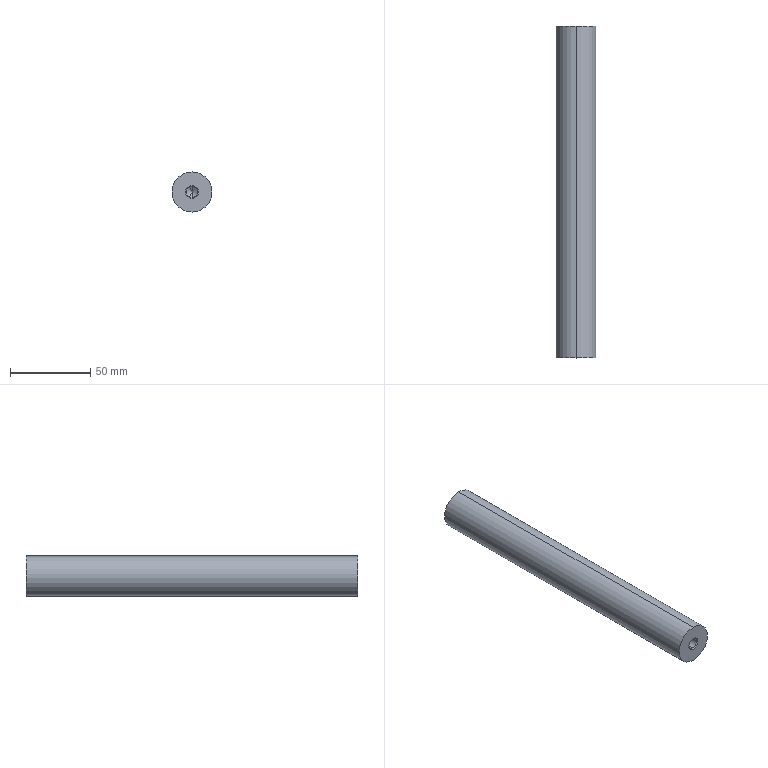Part | STEP file | A14-051 | 1 solid | 16 faces | box 25 x 207 x 25 mm | volume 99936 mm3 | cone 8 | cylinder 6 | plane 2 | commonest cylinder face diameters 6.8 x4 25 x2
STEP:
#1=CARTESIAN_POINT('',(0.,0.,0.));
#2=DIRECTION('',(0.,0.,1.));
#3=DIRECTION('',(1.,0.,0.));
#4=AXIS2_PLACEMENT_3D('',#1,#2,#3);
#5=CARTESIAN_POINT('',(0.,102.875,3.4));
#6=VERTEX_POINT('',#5);
#7=CARTESIAN_POINT('',(0.,103.5,4.025));
#8=VERTEX_POINT('',#7);
#9=CARTESIAN_POINT('',(0.,103.5,4.025));
#10=DIRECTION('',(0.,0.7071,0.7071));
#11=VECTOR('',#10,1.);
#12=LINE('',#9,#11);
#13=CARTESIAN_POINT('',(0.,103.5,0.));
#14=DIRECTION('',(0.,1.,0.));
#15=DIRECTION('',(0.,0.,1.));
#16=AXIS2_PLACEMENT_3D('',#13,#14,#15);
#17=CONICAL_SURFACE('',#16,4.025,0.7854);
#18=CARTESIAN_POINT('',(6.283,0.));
#19=DIRECTION('',(0.,1.));
#20=VECTOR('',#19,1.);
#21=LINE('',#18,#20);
#22=(GEOMETRIC_REPRESENTATION_CONTEXT(2)PARAMETRIC_REPRESENTATION_CONTEXT()REPRESENTATION_CONTEXT('',''));
#23=DEFINITIONAL_REPRESENTATION('',(#21),#22);
#24=PCURVE('',#17,#23);
#25=CARTESIAN_POINT('',(0.,103.5,0.));
#26=DIRECTION('',(0.,1.,0.));
#27=DIRECTION('',(0.,0.,1.));
#28=AXIS2_PLACEMENT_3D('',#25,#26,#27);
#29=CONICAL_SURFACE('',#28,4.025,0.7854);
#30=CARTESIAN_POINT('',(0.,0.));
#31=DIRECTION('',(0.,1.));
#32=VECTOR('',#31,1.);
#33=LINE('',#30,#32);
#34=(GEOMETRIC_REPRESENTATION_CONTEXT(2)PARAMETRIC_REPRESENTATION_CONTEXT()REPRESENTATION_CONTEXT('',''));
#35=DEFINITIONAL_REPRESENTATION('',(#33),#34);
#36=PCURVE('',#29,#35);
#37=SURFACE_CURVE('',#12,(#24,#36),.PCURVE_S1.);
#38=EDGE_CURVE('',#6,#8,#37,.T.);
#39=ORIENTED_EDGE('',*,*,#38,.T.);
#40=CARTESIAN_POINT('',(0.,103.5,-4.025));
#41=VERTEX_POINT('',#40);
#42=CARTESIAN_POINT('',(0.,103.5,0.));
#43=DIRECTION('',(0.,1.,0.));
#44=DIRECTION('',(0.,0.,1.));
#45=AXIS2_PLACEMENT_3D('',#42,#43,#44);
#46=CIRCLE('',#45,4.025);
#47=CARTESIAN_POINT('',(0.,0.));
#48=DIRECTION('',(1.,0.));
#49=VECTOR('',#48,1.);
#50=LINE('',#47,#49);
#51=(GEOMETRIC_REPRESENTATION_CONTEXT(2)PARAMETRIC_REPRESENTATION_CONTEXT()REPRESENTATION_CONTEXT('',''));
#52=DEFINITIONAL_REPRESENTATION('',(#50),#51);
#53=PCURVE('',#17,#52);
#54=CARTESIAN_POINT('',(0.,103.5,0.));
#55=DIRECTION('',(0.,1.,0.));
#56=DIRECTION('',(0.,0.,1.));
#57=AXIS2_PLACEMENT_3D('',#54,#55,#56);
#58=PLANE('',#57);
#59=CARTESIAN_POINT('',(0.,0.));
#60=DIRECTION('',(1.,0.));
#61=AXIS2_PLACEMENT_2D('',#59,#60);
#62=CIRCLE('',#61,4.025);
#63=(GEOMETRIC_REPRESENTATION_CONTEXT(2)PARAMETRIC_REPRESENTATION_CONTEXT()REPRESENTATION_CONTEXT('',''));
#64=DEFINITIONAL_REPRESENTATION('',(#62),#63);
#65=PCURVE('',#58,#64);
#66=SURFACE_CURVE('',#46,(#53,#65),.PCURVE_S1.);
#67=EDGE_CURVE('',#41,#8,#66,.T.);
#68=ORIENTED_EDGE('',*,*,#67,.F.);
#69=CARTESIAN_POINT('',(0.,102.875,-3.4));
#70=VERTEX_POINT('',#69);
#71=CARTESIAN_POINT('',(0.,103.5,-4.025));
#72=DIRECTION('',(0.,0.7071,-0.7071));
#73=VECTOR('',#72,1.);
#74=LINE('',#71,#73);
#75=CARTESIAN_POINT('',(3.142,0.));
#76=DIRECTION('',(0.,1.));
#77=VECTOR('',#76,1.);
#78=LINE('',#75,#77);
#79=(GEOMETRIC_REPRESENTATION_CONTEXT(2)PARAMETRIC_REPRESENTATION_CONTEXT()REPRESENTATION_CONTEXT('',''));
#80=DEFINITIONAL_REPRESENTATION('',(#78),#79);
#81=PCURVE('',#17,#80);
#82=CARTESIAN_POINT('',(3.142,0.));
#83=DIRECTION('',(0.,1.));
#84=VECTOR('',#83,1.);
#85=LINE('',#82,#84);
#86=(GEOMETRIC_REPRESENTATION_CONTEXT(2)PARAMETRIC_REPRESENTATION_CONTEXT()REPRESENTATION_CONTEXT('',''));
#87=DEFINITIONAL_REPRESENTATION('',(#85),#86);
#88=PCURVE('',#29,#87);
#89=SURFACE_CURVE('',#74,(#81,#88),.PCURVE_S1.);
#90=EDGE_CURVE('',#70,#41,#89,.T.);
#91=ORIENTED_EDGE('',*,*,#90,.F.);
#92=CARTESIAN_POINT('',(0.,102.875,0.));
#93=DIRECTION('',(0.,1.,0.));
#94=DIRECTION('',(0.,0.,1.));
#95=AXIS2_PLACEMENT_3D('',#92,#93,#94);
#96=CIRCLE('',#95,3.4);
#97=CARTESIAN_POINT('',(0.,-0.625));
#98=DIRECTION('',(1.,0.));
#99=VECTOR('',#98,1.);
#100=LINE('',#97,#99);
#101=(GEOMETRIC_REPRESENTATION_CONTEXT(2)PARAMETRIC_REPRESENTATION_CONTEXT()REPRESENTATION_CONTEXT('',''));
#102=DEFINITIONAL_REPRESENTATION('',(#100),#101);
#103=PCURVE('',#17,#102);
#104=CARTESIAN_POINT('',(0.,103.5,0.));
#105=DIRECTION('',(0.,1.,0.));
#106=DIRECTION('',(0.,0.,1.));
#107=AXIS2_PLACEMENT_3D('',#104,#105,#106);
#108=CYLINDRICAL_SURFACE('',#107,3.4);
#109=CARTESIAN_POINT('',(0.,-0.625));
#110=DIRECTION('',(1.,0.));
#111=VECTOR('',#110,1.);
#112=LINE('',#109,#111);
#113=(GEOMETRIC_REPRESENTATION_CONTEXT(2)PARAMETRIC_REPRESENTATION_CONTEXT()REPRESENTATION_CONTEXT('',''));
#114=DEFINITIONAL_REPRESENTATION('',(#112),#113);
#115=PCURVE('',#108,#114);
#116=SURFACE_CURVE('',#96,(#103,#115),.PCURVE_S1.);
#117=EDGE_CURVE('',#70,#6,#116,.T.);
#118=ORIENTED_EDGE('',*,*,#117,.T.);
#119=EDGE_LOOP('',(#39,#68,#91,#118));
#120=FACE_BOUND('',#119,.F.);
#121=ADVANCED_FACE('',(#120),#17,.F.);
#122=CARTESIAN_POINT('',(0.,81.25,3.4));
#123=VERTEX_POINT('',#122);
#124=CARTESIAN_POINT('',(0.,103.5,3.4));
#125=DIRECTION('',(0.,1.,0.));
#126=VECTOR('',#125,1.);
#127=LINE('',#124,#126);
#128=CARTESIAN_POINT('',(6.283,0.));
#129=DIRECTION('',(0.,1.));
#130=VECTOR('',#129,1.);
#131=LINE('',#128,#130);
#132=(GEOMETRIC_REPRESENTATION_CONTEXT(2)PARAMETRIC_REPRESENTATION_CONTEXT()REPRESENTATION_CONTEXT('',''));
#133=DEFINITIONAL_REPRESENTATION('',(#131),#132);
#134=PCURVE('',#108,#133);
#135=CARTESIAN_POINT('',(0.,103.5,0.));
#136=DIRECTION('',(0.,1.,0.));
#137=DIRECTION('',(0.,0.,1.));
#138=AXIS2_PLACEMENT_3D('',#135,#136,#137);
#139=CYLINDRICAL_SURFACE('',#138,3.4);
#140=CARTESIAN_POINT('',(0.,0.));
#141=DIRECTION('',(0.,1.));
#142=VECTOR('',#141,1.);
#143=LINE('',#140,#142);
#144=(GEOMETRIC_REPRESENTATION_CONTEXT(2)PARAMETRIC_REPRESENTATION_CONTEXT()REPRESENTATION_CONTEXT('',''));
#145=DEFINITIONAL_REPRESENTATION('',(#143),#144);
#146=PCURVE('',#139,#145);
#147=SURFACE_CURVE('',#127,(#134,#146),.PCURVE_S1.);
#148=EDGE_CURVE('',#123,#6,#147,.T.);
#149=ORIENTED_EDGE('',*,*,#148,.T.);
#150=ORIENTED_EDGE('',*,*,#117,.F.);
#151=CARTESIAN_POINT('',(0.,81.25,-3.4));
#152=VERTEX_POINT('',#151);
#153=CARTESIAN_POINT('',(0.,103.5,-3.4));
#154=DIRECTION('',(0.,1.,0.));
#155=VECTOR('',#154,1.);
#156=LINE('',#153,#155);
#157=CARTESIAN_POINT('',(3.142,0.));
#158=DIRECTION('',(0.,1.));
#159=VECTOR('',#158,1.);
#160=LINE('',#157,#159);
#161=(GEOMETRIC_REPRESENTATION_CONTEXT(2)PARAMETRIC_REPRESENTATION_CONTEXT()REPRESENTATION_CONTEXT('',''));
#162=DEFINITIONAL_REPRESENTATION('',(#160),#161);
#163=PCURVE('',#108,#162);
#164=CARTESIAN_POINT('',(3.142,0.));
#165=DIRECTION('',(0.,1.));
#166=VECTOR('',#165,1.);
#167=LINE('',#164,#166);
#168=(GEOMETRIC_REPRESENTATION_CONTEXT(2)PARAMETRIC_REPRESENTATION_CONTEXT()REPRESENTATION_CONTEXT('',''));
#169=DEFINITIONAL_REPRESENTATION('',(#167),#168);
#170=PCURVE('',#139,#169);
#171=SURFACE_CURVE('',#156,(#163,#170),.PCURVE_S1.);
#172=EDGE_CURVE('',#152,#70,#171,.T.);
#173=ORIENTED_EDGE('',*,*,#172,.F.);
#174=CARTESIAN_POINT('',(0.,81.25,0.));
#175=DIRECTION('',(0.,1.,0.));
#176=DIRECTION('',(0.,0.,1.));
#177=AXIS2_PLACEMENT_3D('',#174,#175,#176);
#178=CIRCLE('',#177,3.4);
#179=CARTESIAN_POINT('',(0.,-22.25));
#180=DIRECTION('',(1.,0.));
#181=VECTOR('',#180,1.);
#182=LINE('',#179,#181);
#183=(GEOMETRIC_REPRESENTATION_CONTEXT(2)PARAMETRIC_REPRESENTATION_CONTEXT()REPRESENTATION_CONTEXT('',''));
#184=DEFINITIONAL_REPRESENTATION('',(#182),#183);
#185=PCURVE('',#108,#184);
#186=CARTESIAN_POINT('',(0.,81.25,0.));
#187=DIRECTION('',(0.,1.,0.));
#188=DIRECTION('',(0.,0.,1.));
#189=AXIS2_PLACEMENT_3D('',#186,#187,#188);
#190=CONICAL_SURFACE('',#189,3.4,1.03);
#191=CARTESIAN_POINT('',(0.,0.));
#192=DIRECTION('',(1.,0.));
#193=VECTOR('',#192,1.);
#194=LINE('',#191,#193);
#195=(GEOMETRIC_REPRESENTATION_CONTEXT(2)PARAMETRIC_REPRESENTATION_CONTEXT()REPRESENTATION_CONTEXT('',''));
#196=DEFINITIONAL_REPRESENTATION('',(#194),#195);
#197=PCURVE('',#190,#196);
#198=SURFACE_CURVE('',#178,(#185,#197),.PCURVE_S1.);
#199=EDGE_CURVE('',#152,#123,#198,.T.);
#200=ORIENTED_EDGE('',*,*,#199,.T.);
#201=EDGE_LOOP('',(#149,#150,#173,#200));
#202=FACE_BOUND('',#201,.F.);
#203=ADVANCED_FACE('',(#202),#108,.F.);
#204=ORIENTED_EDGE('',*,*,#199,.F.);
#205=CARTESIAN_POINT('',(0.,79.207,0.));
#206=VERTEX_POINT('',#205);
#207=CARTESIAN_POINT('',(0.,81.25,-3.4));
#208=DIRECTION('',(0.,0.515,-0.8572));
#209=VECTOR('',#208,1.);
#210=LINE('',#207,#209);
#211=CARTESIAN_POINT('',(3.142,-2.043));
#212=CARTESIAN_POINT('',(3.142,-2.012));
#213=CARTESIAN_POINT('',(3.142,-1.95));
#214=CARTESIAN_POINT('',(3.142,-1.857));
#215=CARTESIAN_POINT('',(3.142,-1.764));
#216=CARTESIAN_POINT('',(3.142,-1.671));
#217=CARTESIAN_POINT('',(3.142,-1.579));
#218=CARTESIAN_POINT('',(3.142,-1.486));
#219=CARTESIAN_POINT('',(3.142,-1.393));
#220=CARTESIAN_POINT('',(3.142,-1.3));
#221=CARTESIAN_POINT('',(3.142,-1.207));
#222=CARTESIAN_POINT('',(3.142,-1.114));
#223=CARTESIAN_POINT('',(3.142,-1.021));
#224=CARTESIAN_POINT('',(3.142,-0.9286));
#225=CARTESIAN_POINT('',(3.142,-0.8357));
#226=CARTESIAN_POINT('',(3.142,-0.7429));
#227=CARTESIAN_POINT('',(3.142,-0.65));
#228=CARTESIAN_POINT('',(3.142,-0.5572));
#229=CARTESIAN_POINT('',(3.142,-0.4643));
#230=CARTESIAN_POINT('',(3.142,-0.3714));
#231=CARTESIAN_POINT('',(3.142,-0.2786));
#232=CARTESIAN_POINT('',(3.142,-0.1857));
#233=CARTESIAN_POINT('',(3.142,-0.09286));
#234=CARTESIAN_POINT('',(3.142,-0.03095));
#235=CARTESIAN_POINT('',(3.142,0.));
#236=B_SPLINE_CURVE_WITH_KNOTS('',3,(#211,#212,#213,#214,#215,#216,#217,#218,#219,#220,#221,#222,#223,#224,#225,#226,#227,#228,#229,#230,#231,#232,#233,#234,#235),.UNSPECIFIED.,.F.,.F.,(4,1,1,1,1,1,1,1,1,1,1,1,1,1,1,1,1,1,1,1,1,1,4),(-3.967,-3.786,-3.606,-3.426,-3.245,-3.065,-2.885,-2.704,-2.524,-2.344,-2.164,-1.983,-1.803,-1.623,-1.442,-1.262,-1.082,-0.9015,-0.7212,-0.5409,-0.3606,-0.1803,0.),.UNSPECIFIED.);
#237=(GEOMETRIC_REPRESENTATION_CONTEXT(2)PARAMETRIC_REPRESENTATION_CONTEXT()REPRESENTATION_CONTEXT('',''));
#238=DEFINITIONAL_REPRESENTATION('',(#236),#237);
#239=PCURVE('',#190,#238);
#240=CARTESIAN_POINT('',(0.,81.25,0.));
#241=DIRECTION('',(0.,1.,0.));
#242=DIRECTION('',(0.,0.,1.));
#243=AXIS2_PLACEMENT_3D('',#240,#241,#242);
#244=CONICAL_SURFACE('',#243,3.4,1.03);
#245=CARTESIAN_POINT('',(3.142,-2.043));
#246=CARTESIAN_POINT('',(3.142,-2.012));
#247=CARTESIAN_POINT('',(3.142,-1.95));
#248=CARTESIAN_POINT('',(3.142,-1.857));
#249=CARTESIAN_POINT('',(3.142,-1.764));
#250=CARTESIAN_POINT('',(3.142,-1.671));
#251=CARTESIAN_POINT('',(3.142,-1.579));
#252=CARTESIAN_POINT('',(3.142,-1.486));
#253=CARTESIAN_POINT('',(3.142,-1.393));
#254=CARTESIAN_POINT('',(3.142,-1.3));
#255=CARTESIAN_POINT('',(3.142,-1.207));
#256=CARTESIAN_POINT('',(3.142,-1.114));
#257=CARTESIAN_POINT('',(3.142,-1.021));
#258=CARTESIAN_POINT('',(3.142,-0.9286));
#259=CARTESIAN_POINT('',(3.142,-0.8357));
#260=CARTESIAN_POINT('',(3.142,-0.7429));
#261=CARTESIAN_POINT('',(3.142,-0.65));
#262=CARTESIAN_POINT('',(3.142,-0.5572));
#263=CARTESIAN_POINT('',(3.142,-0.4643));
#264=CARTESIAN_POINT('',(3.142,-0.3714));
#265=CARTESIAN_POINT('',(3.142,-0.2786));
#266=CARTESIAN_POINT('',(3.142,-0.1857));
#267=CARTESIAN_POINT('',(3.142,-0.09286));
#268=CARTESIAN_POINT('',(3.142,-0.03095));
#269=CARTESIAN_POINT('',(3.142,0.));
#270=B_SPLINE_CURVE_WITH_KNOTS('',3,(#245,#246,#247,#248,#249,#250,#251,#252,#253,#254,#255,#256,#257,#258,#259,#260,#261,#262,#263,#264,#265,#266,#267,#268,#269),.UNSPECIFIED.,.F.,.F.,(4,1,1,1,1,1,1,1,1,1,1,1,1,1,1,1,1,1,1,1,1,1,4),(-3.967,-3.786,-3.606,-3.426,-3.245,-3.065,-2.885,-2.704,-2.524,-2.344,-2.164,-1.983,-1.803,-1.623,-1.442,-1.262,-1.082,-0.9015,-0.7212,-0.5409,-0.3606,-0.1803,0.),.UNSPECIFIED.);
#271=(GEOMETRIC_REPRESENTATION_CONTEXT(2)PARAMETRIC_REPRESENTATION_CONTEXT()REPRESENTATION_CONTEXT('',''));
#272=DEFINITIONAL_REPRESENTATION('',(#270),#271);
#273=PCURVE('',#244,#272);
#274=SURFACE_CURVE('',#210,(#239,#273),.PCURVE_S1.);
#275=EDGE_CURVE('',#206,#152,#274,.T.);
#276=ORIENTED_EDGE('',*,*,#275,.F.);
#277=CARTESIAN_POINT('',(0.,81.25,3.4));
#278=DIRECTION('',(0.,0.515,0.8572));
#279=VECTOR('',#278,1.);
#280=LINE('',#277,#279);
#281=CARTESIAN_POINT('',(6.283,-2.043));
#282=CARTESIAN_POINT('',(6.283,-2.012));
#283=CARTESIAN_POINT('',(6.283,-1.95));
#284=CARTESIAN_POINT('',(6.283,-1.857));
#285=CARTESIAN_POINT('',(6.283,-1.764));
#286=CARTESIAN_POINT('',(6.283,-1.671));
#287=CARTESIAN_POINT('',(6.283,-1.579));
#288=CARTESIAN_POINT('',(6.283,-1.486));
#289=CARTESIAN_POINT('',(6.283,-1.393));
#290=CARTESIAN_POINT('',(6.283,-1.3));
#291=CARTESIAN_POINT('',(6.283,-1.207));
#292=CARTESIAN_POINT('',(6.283,-1.114));
#293=CARTESIAN_POINT('',(6.283,-1.021));
#294=CARTESIAN_POINT('',(6.283,-0.9286));
#295=CARTESIAN_POINT('',(6.283,-0.8357));
#296=CARTESIAN_POINT('',(6.283,-0.7429));
#297=CARTESIAN_POINT('',(6.283,-0.65));
#298=CARTESIAN_POINT('',(6.283,-0.5572));
#299=CARTESIAN_POINT('',(6.283,-0.4643));
#300=CARTESIAN_POINT('',(6.283,-0.3714));
#301=CARTESIAN_POINT('',(6.283,-0.2786));
#302=CARTESIAN_POINT('',(6.283,-0.1857));
#303=CARTESIAN_POINT('',(6.283,-0.09286));
#304=CARTESIAN_POINT('',(6.283,-0.03095));
#305=CARTESIAN_POINT('',(6.283,0.));
#306=B_SPLINE_CURVE_WITH_KNOTS('',3,(#281,#282,#283,#284,#285,#286,#287,#288,#289,#290,#291,#292,#293,#294,#295,#296,#297,#298,#299,#300,#301,#302,#303,#304,#305),.UNSPECIFIED.,.F.,.F.,(4,1,1,1,1,1,1,1,1,1,1,1,1,1,1,1,1,1,1,1,1,1,4),(-3.967,-3.786,-3.606,-3.426,-3.245,-3.065,-2.885,-2.704,-2.524,-2.344,-2.164,-1.983,-1.803,-1.623,-1.442,-1.262,-1.082,-0.9015,-0.7212,-0.5409,-0.3606,-0.1803,0.),.UNSPECIFIED.);
#307=(GEOMETRIC_REPRESENTATION_CONTEXT(2)PARAMETRIC_REPRESENTATION_CONTEXT()REPRESENTATION_CONTEXT('',''));
#308=DEFINITIONAL_REPRESENTATION('',(#306),#307);
#309=PCURVE('',#190,#308);
#310=CARTESIAN_POINT('',(0.,-2.043));
#311=CARTESIAN_POINT('',(0.,-2.012));
#312=CARTESIAN_POINT('',(0.,-1.95));
#313=CARTESIAN_POINT('',(0.,-1.857));
#314=CARTESIAN_POINT('',(0.,-1.764));
#315=CARTESIAN_POINT('',(0.,-1.671));
#316=CARTESIAN_POINT('',(0.,-1.579));
#317=CARTESIAN_POINT('',(0.,-1.486));
#318=CARTESIAN_POINT('',(0.,-1.393));
#319=CARTESIAN_POINT('',(0.,-1.3));
#320=CARTESIAN_POINT('',(0.,-1.207));
#321=CARTESIAN_POINT('',(0.,-1.114));
#322=CARTESIAN_POINT('',(0.,-1.021));
#323=CARTESIAN_POINT('',(0.,-0.9286));
#324=CARTESIAN_POINT('',(0.,-0.8357));
#325=CARTESIAN_POINT('',(0.,-0.7429));
#326=CARTESIAN_POINT('',(0.,-0.65));
#327=CARTESIAN_POINT('',(0.,-0.5572));
#328=CARTESIAN_POINT('',(0.,-0.4643));
#329=CARTESIAN_POINT('',(0.,-0.3714));
#330=CARTESIAN_POINT('',(0.,-0.2786));
#331=CARTESIAN_POINT('',(0.,-0.1857));
#332=CARTESIAN_POINT('',(0.,-0.09286));
#333=CARTESIAN_POINT('',(0.,-0.03095));
#334=CARTESIAN_POINT('',(0.,0.));
#335=B_SPLINE_CURVE_WITH_KNOTS('',3,(#310,#311,#312,#313,#314,#315,#316,#317,#318,#319,#320,#321,#322,#323,#324,#325,#326,#327,#328,#329,#330,#331,#332,#333,#334),.UNSPECIFIED.,.F.,.F.,(4,1,1,1,1,1,1,1,1,1,1,1,1,1,1,1,1,1,1,1,1,1,4),(-3.967,-3.786,-3.606,-3.426,-3.245,-3.065,-2.885,-2.704,-2.524,-2.344,-2.164,-1.983,-1.803,-1.623,-1.442,-1.262,-1.082,-0.9015,-0.7212,-0.5409,-0.3606,-0.1803,0.),.UNSPECIFIED.);
#336=(GEOMETRIC_REPRESENTATION_CONTEXT(2)PARAMETRIC_REPRESENTATION_CONTEXT()REPRESENTATION_CONTEXT('',''));
#337=DEFINITIONAL_REPRESENTATION('',(#335),#336);
#338=PCURVE('',#244,#337);
#339=SURFACE_CURVE('',#280,(#309,#338),.PCURVE_S1.);
#340=EDGE_CURVE('',#206,#123,#339,.T.);
#341=ORIENTED_EDGE('',*,*,#340,.T.);
#342=EDGE_LOOP('',(#204,#276,#341));
#343=FACE_BOUND('',#342,.F.);
#344=ADVANCED_FACE('',(#343),#190,.F.);
#345=CARTESIAN_POINT('',(0.,-102.875,-3.4));
#346=VERTEX_POINT('',#345);
#347=CARTESIAN_POINT('',(0.,-103.5,-4.025));
#348=VERTEX_POINT('',#347);
#349=CARTESIAN_POINT('',(0.,-103.5,-4.025));
#350=DIRECTION('',(0.,-0.7071,-0.7071));
#351=VECTOR('',#350,1.);
#352=LINE('',#349,#351);
#353=CARTESIAN_POINT('',(0.,-103.5,0.));
#354=DIRECTION('',(0.,-1.,0.));
#355=DIRECTION('',(0.,0.,-1.));
#356=AXIS2_PLACEMENT_3D('',#353,#354,#355);
#357=CONICAL_SURFACE('',#356,4.025,0.7854);
#358=CARTESIAN_POINT('',(6.283,0.));
#359=DIRECTION('',(0.,1.));
#360=VECTOR('',#359,1.);
#361=LINE('',#358,#360);
#362=(GEOMETRIC_REPRESENTATION_CONTEXT(2)PARAMETRIC_REPRESENTATION_CONTEXT()REPRESENTATION_CONTEXT('',''));
#363=DEFINITIONAL_REPRESENTATION('',(#361),#362);
#364=PCURVE('',#357,#363);
#365=CARTESIAN_POINT('',(0.,-103.5,0.));
#366=DIRECTION('',(0.,-1.,0.));
#367=DIRECTION('',(0.,0.,-1.));
#368=AXIS2_PLACEMENT_3D('',#365,#366,#367);
#369=CONICAL_SURFACE('',#368,4.025,0.7854);
#370=CARTESIAN_POINT('',(0.,0.));
#371=DIRECTION('',(0.,1.));
#372=VECTOR('',#371,1.);
#373=LINE('',#370,#372);
#374=(GEOMETRIC_REPRESENTATION_CONTEXT(2)PARAMETRIC_REPRESENTATION_CONTEXT()REPRESENTATION_CONTEXT('',''));
#375=DEFINITIONAL_REPRESENTATION('',(#373),#374);
#376=PCURVE('',#369,#375);
#377=SURFACE_CURVE('',#352,(#364,#376),.PCURVE_S1.);
#378=EDGE_CURVE('',#346,#348,#377,.T.);
#379=ORIENTED_EDGE('',*,*,#378,.T.);
#380=CARTESIAN_POINT('',(0.,-103.5,4.025));
#381=VERTEX_POINT('',#380);
#382=CARTESIAN_POINT('',(0.,-103.5,0.));
#383=DIRECTION('',(0.,-1.,0.));
#384=DIRECTION('',(0.,0.,-1.));
#385=AXIS2_PLACEMENT_3D('',#382,#383,#384);
#386=CIRCLE('',#385,4.025);
#387=CARTESIAN_POINT('',(0.,0.));
#388=DIRECTION('',(1.,0.));
#389=VECTOR('',#388,1.);
#390=LINE('',#387,#389);
#391=(GEOMETRIC_REPRESENTATION_CONTEXT(2)PARAMETRIC_REPRESENTATION_CONTEXT()REPRESENTATION_CONTEXT('',''));
#392=DEFINITIONAL_REPRESENTATION('',(#390),#391);
#393=PCURVE('',#357,#392);
#394=CARTESIAN_POINT('',(0.,-103.5,0.));
#395=DIRECTION('',(0.,1.,0.));
#396=DIRECTION('',(0.,0.,1.));
#397=AXIS2_PLACEMENT_3D('',#394,#395,#396);
#398=PLANE('',#397);
#399=CARTESIAN_POINT('',(-4.025,0.));
#400=CARTESIAN_POINT('',(-4.025,6.972));
#401=CARTESIAN_POINT('',(2.013,3.486));
#402=CARTESIAN_POINT('',(8.05,0.));
#403=CARTESIAN_POINT('',(2.013,-3.486));
#404=CARTESIAN_POINT('',(-4.025,-6.972));
#405=CARTESIAN_POINT('',(-4.025,0.));
#406=(BOUNDED_CURVE()B_SPLINE_CURVE(2,(#399,#400,#401,#402,#403,#404,#405),.UNSPECIFIED.,.T.,.F.)B_SPLINE_CURVE_WITH_KNOTS((1,2,2,2,2,1),(-2.094,0.,2.094,4.189,6.283,8.378),.UNSPECIFIED.)CURVE()GEOMETRIC_REPRESENTATION_ITEM()RATIONAL_B_SPLINE_CURVE((1.,0.5,1.,0.5,1.,0.5,1.))REPRESENTATION_ITEM(''));
#407=(GEOMETRIC_REPRESENTATION_CONTEXT(2)PARAMETRIC_REPRESENTATION_CONTEXT()REPRESENTATION_CONTEXT('',''));
#408=DEFINITIONAL_REPRESENTATION('',(#406),#407);
#409=PCURVE('',#398,#408);
#410=SURFACE_CURVE('',#386,(#393,#409),.PCURVE_S1.);
#411=EDGE_CURVE('',#381,#348,#410,.T.);
#412=ORIENTED_EDGE('',*,*,#411,.F.);
#413=CARTESIAN_POINT('',(0.,-102.875,3.4));
#414=VERTEX_POINT('',#413);
#415=CARTESIAN_POINT('',(0.,-103.5,4.025));
#416=DIRECTION('',(0.,-0.7071,0.7071));
#417=VECTOR('',#416,1.);
#418=LINE('',#415,#417);
#419=CARTESIAN_POINT('',(3.142,0.));
#420=DIRECTION('',(0.,1.));
#421=VECTOR('',#420,1.);
#422=LINE('',#419,#421);
#423=(GEOMETRIC_REPRESENTATION_CONTEXT(2)PARAMETRIC_REPRESENTATION_CONTEXT()REPRESENTATION_CONTEXT('',''));
#424=DEFINITIONAL_REPRESENTATION('',(#422),#423);
#425=PCURVE('',#357,#424);
#426=CARTESIAN_POINT('',(3.142,0.));
#427=DIRECTION('',(0.,1.));
#428=VECTOR('',#427,1.);
#429=LINE('',#426,#428);
#430=(GEOMETRIC_REPRESENTATION_CONTEXT(2)PARAMETRIC_REPRESENTATION_CONTEXT()REPRESENTATION_CONTEXT('',''));
#431=DEFINITIONAL_REPRESENTATION('',(#429),#430);
#432=PCURVE('',#369,#431);
#433=SURFACE_CURVE('',#418,(#425,#432),.PCURVE_S1.);
#434=EDGE_CURVE('',#414,#381,#433,.T.);
#435=ORIENTED_EDGE('',*,*,#434,.F.);
#436=CARTESIAN_POINT('',(0.,-102.875,0.));
#437=DIRECTION('',(0.,-1.,0.));
#438=DIRECTION('',(0.,0.,-1.));
#439=AXIS2_PLACEMENT_3D('',#436,#437,#438);
#440=CIRCLE('',#439,3.4);
#441=CARTESIAN_POINT('',(0.,-0.625));
#442=DIRECTION('',(1.,0.));
#443=VECTOR('',#442,1.);
#444=LINE('',#441,#443);
#445=(GEOMETRIC_REPRESENTATION_CONTEXT(2)PARAMETRIC_REPRESENTATION_CONTEXT()REPRESENTATION_CONTEXT('',''));
#446=DEFINITIONAL_REPRESENTATION('',(#444),#445);
#447=PCURVE('',#357,#446);
#448=CARTESIAN_POINT('',(0.,-103.5,0.));
#449=DIRECTION('',(0.,-1.,0.));
#450=DIRECTION('',(0.,0.,-1.));
#451=AXIS2_PLACEMENT_3D('',#448,#449,#450);
#452=CYLINDRICAL_SURFACE('',#451,3.4);
#453=CARTESIAN_POINT('',(0.,-0.625));
#454=DIRECTION('',(1.,0.));
#455=VECTOR('',#454,1.);
#456=LINE('',#453,#455);
#457=(GEOMETRIC_REPRESENTATION_CONTEXT(2)PARAMETRIC_REPRESENTATION_CONTEXT()REPRESENTATION_CONTEXT('',''));
#458=DEFINITIONAL_REPRESENTATION('',(#456),#457);
#459=PCURVE('',#452,#458);
#460=SURFACE_CURVE('',#440,(#447,#459),.PCURVE_S1.);
#461=EDGE_CURVE('',#414,#346,#460,.T.);
#462=ORIENTED_EDGE('',*,*,#461,.T.);
#463=EDGE_LOOP('',(#379,#412,#435,#462));
#464=FACE_BOUND('',#463,.F.);
#465=ADVANCED_FACE('',(#464),#357,.F.);
#466=CARTESIAN_POINT('',(0.,-81.25,-3.4));
#467=VERTEX_POINT('',#466);
#468=CARTESIAN_POINT('',(0.,-103.5,-3.4));
#469=DIRECTION('',(0.,-1.,0.));
#470=VECTOR('',#469,1.);
#471=LINE('',#468,#470);
#472=CARTESIAN_POINT('',(6.283,0.));
#473=DIRECTION('',(0.,1.));
#474=VECTOR('',#473,1.);
#475=LINE('',#472,#474);
#476=(GEOMETRIC_REPRESENTATION_CONTEXT(2)PARAMETRIC_REPRESENTATION_CONTEXT()REPRESENTATION_CONTEXT('',''));
#477=DEFINITIONAL_REPRESENTATION('',(#475),#476);
#478=PCURVE('',#452,#477);
#479=CARTESIAN_POINT('',(0.,-103.5,0.));
#480=DIRECTION('',(0.,-1.,0.));
#481=DIRECTION('',(0.,0.,-1.));
#482=AXIS2_PLACEMENT_3D('',#479,#480,#481);
#483=CYLINDRICAL_SURFACE('',#482,3.4);
#484=CARTESIAN_POINT('',(0.,0.));
#485=DIRECTION('',(0.,1.));
#486=VECTOR('',#485,1.);
#487=LINE('',#484,#486);
#488=(GEOMETRIC_REPRESENTATION_CONTEXT(2)PARAMETRIC_REPRESENTATION_CONTEXT()REPRESENTATION_CONTEXT('',''));
#489=DEFINITIONAL_REPRESENTATION('',(#487),#488);
#490=PCURVE('',#483,#489);
#491=SURFACE_CURVE('',#471,(#478,#490),.PCURVE_S1.);
#492=EDGE_CURVE('',#467,#346,#491,.T.);
#493=ORIENTED_EDGE('',*,*,#492,.T.);
#494=ORIENTED_EDGE('',*,*,#461,.F.);
#495=CARTESIAN_POINT('',(0.,-81.25,3.4));
#496=VERTEX_POINT('',#495);
#497=CARTESIAN_POINT('',(0.,-103.5,3.4));
#498=DIRECTION('',(0.,-1.,0.));
#499=VECTOR('',#498,1.);
#500=LINE('',#497,#499);
#501=CARTESIAN_POINT('',(3.142,0.));
#502=DIRECTION('',(0.,1.));
#503=VECTOR('',#502,1.);
#504=LINE('',#501,#503);
#505=(GEOMETRIC_REPRESENTATION_CONTEXT(2)PARAMETRIC_REPRESENTATION_CONTEXT()REPRESENTATION_CONTEXT('',''));
#506=DEFINITIONAL_REPRESENTATION('',(#504),#505);
#507=PCURVE('',#452,#506);
#508=CARTESIAN_POINT('',(3.142,0.));
#509=DIRECTION('',(0.,1.));
#510=VECTOR('',#509,1.);
#511=LINE('',#508,#510);
#512=(GEOMETRIC_REPRESENTATION_CONTEXT(2)PARAMETRIC_REPRESENTATION_CONTEXT()REPRESENTATION_CONTEXT('',''));
#513=DEFINITIONAL_REPRESENTATION('',(#511),#512);
#514=PCURVE('',#483,#513);
#515=SURFACE_CURVE('',#500,(#507,#514),.PCURVE_S1.);
#516=EDGE_CURVE('',#496,#414,#515,.T.);
#517=ORIENTED_EDGE('',*,*,#516,.F.);
#518=CARTESIAN_POINT('',(0.,-81.25,0.));
#519=DIRECTION('',(0.,-1.,0.));
#520=DIRECTION('',(0.,0.,-1.));
#521=AXIS2_PLACEMENT_3D('',#518,#519,#520);
#522=CIRCLE('',#521,3.4);
#523=CARTESIAN_POINT('',(0.,-22.25));
#524=DIRECTION('',(1.,0.));
#525=VECTOR('',#524,1.);
#526=LINE('',#523,#525);
#527=(GEOMETRIC_REPRESENTATION_CONTEXT(2)PARAMETRIC_REPRESENTATION_CONTEXT()REPRESENTATION_CONTEXT('',''));
#528=DEFINITIONAL_REPRESENTATION('',(#526),#527);
#529=PCURVE('',#452,#528);
#530=CARTESIAN_POINT('',(0.,-81.25,0.));
#531=DIRECTION('',(0.,-1.,0.));
#532=DIRECTION('',(0.,0.,-1.));
#533=AXIS2_PLACEMENT_3D('',#530,#531,#532);
#534=CONICAL_SURFACE('',#533,3.4,1.03);
#535=CARTESIAN_POINT('',(0.,0.));
#536=DIRECTION('',(1.,0.));
#537=VECTOR('',#536,1.);
#538=LINE('',#535,#537);
#539=(GEOMETRIC_REPRESENTATION_CONTEXT(2)PARAMETRIC_REPRESENTATION_CONTEXT()REPRESENTATION_CONTEXT('',''));
#540=DEFINITIONAL_REPRESENTATION('',(#538),#539);
#541=PCURVE('',#534,#540);
#542=SURFACE_CURVE('',#522,(#529,#541),.PCURVE_S1.);
#543=EDGE_CURVE('',#496,#467,#542,.T.);
#544=ORIENTED_EDGE('',*,*,#543,.T.);
#545=EDGE_LOOP('',(#493,#494,#517,#544));
#546=FACE_BOUND('',#545,.F.);
#547=ADVANCED_FACE('',(#546),#452,.F.);
#548=ORIENTED_EDGE('',*,*,#543,.F.);
#549=CARTESIAN_POINT('',(0.,-79.207,0.));
#550=VERTEX_POINT('',#549);
#551=CARTESIAN_POINT('',(0.,-81.25,3.4));
#552=DIRECTION('',(0.,-0.515,0.8572));
#553=VECTOR('',#552,1.);
#554=LINE('',#551,#553);
#555=CARTESIAN_POINT('',(3.142,-2.043));
#556=CARTESIAN_POINT('',(3.142,-2.012));
#557=CARTESIAN_POINT('',(3.142,-1.95));
#558=CARTESIAN_POINT('',(3.142,-1.857));
#559=CARTESIAN_POINT('',(3.142,-1.764));
#560=CARTESIAN_POINT('',(3.142,-1.671));
#561=CARTESIAN_POINT('',(3.142,-1.579));
#562=CARTESIAN_POINT('',(3.142,-1.486));
#563=CARTESIAN_POINT('',(3.142,-1.393));
#564=CARTESIAN_POINT('',(3.142,-1.3));
#565=CARTESIAN_POINT('',(3.142,-1.207));
#566=CARTESIAN_POINT('',(3.142,-1.114));
#567=CARTESIAN_POINT('',(3.142,-1.021));
#568=CARTESIAN_POINT('',(3.142,-0.9286));
#569=CARTESIAN_POINT('',(3.142,-0.8357));
#570=CARTESIAN_POINT('',(3.142,-0.7429));
#571=CARTESIAN_POINT('',(3.142,-0.65));
#572=CARTESIAN_POINT('',(3.142,-0.5572));
#573=CARTESIAN_POINT('',(3.142,-0.4643));
#574=CARTESIAN_POINT('',(3.142,-0.3714));
#575=CARTESIAN_POINT('',(3.142,-0.2786));
#576=CARTESIAN_POINT('',(3.142,-0.1857));
#577=CARTESIAN_POINT('',(3.142,-0.09286));
#578=CARTESIAN_POINT('',(3.142,-0.03095));
#579=CARTESIAN_POINT('',(3.142,0.));
#580=B_SPLINE_CURVE_WITH_KNOTS('',3,(#555,#556,#557,#558,#559,#560,#561,#562,#563,#564,#565,#566,#567,#568,#569,#570,#571,#572,#573,#574,#575,#576,#577,#578,#579),.UNSPECIFIED.,.F.,.F.,(4,1,1,1,1,1,1,1,1,1,1,1,1,1,1,1,1,1,1,1,1,1,4),(-3.967,-3.786,-3.606,-3.426,-3.245,-3.065,-2.885,-2.704,-2.524,-2.344,-2.164,-1.983,-1.803,-1.623,-1.442,-1.262,-1.082,-0.9015,-0.7212,-0.5409,-0.3606,-0.1803,0.),.UNSPECIFIED.);
#581=(GEOMETRIC_REPRESENTATION_CONTEXT(2)PARAMETRIC_REPRESENTATION_CONTEXT()REPRESENTATION_CONTEXT('',''));
#582=DEFINITIONAL_REPRESENTATION('',(#580),#581);
#583=PCURVE('',#534,#582);
#584=CARTESIAN_POINT('',(0.,-81.25,0.));
#585=DIRECTION('',(0.,-1.,0.));
#586=DIRECTION('',(0.,0.,-1.));
#587=AXIS2_PLACEMENT_3D('',#584,#585,#586);
#588=CONICAL_SURFACE('',#587,3.4,1.03);
#589=CARTESIAN_POINT('',(3.142,-2.043));
#590=CARTESIAN_POINT('',(3.142,-2.012));
#591=CARTESIAN_POINT('',(3.142,-1.95));
#592=CARTESIAN_POINT('',(3.142,-1.857));
#593=CARTESIAN_POINT('',(3.142,-1.764));
#594=CARTESIAN_POINT('',(3.142,-1.671));
#595=CARTESIAN_POINT('',(3.142,-1.579));
#596=CARTESIAN_POINT('',(3.142,-1.486));
#597=CARTESIAN_POINT('',(3.142,-1.393));
#598=CARTESIAN_POINT('',(3.142,-1.3));
#599=CARTESIAN_POINT('',(3.142,-1.207));
#600=CARTESIAN_POINT('',(3.142,-1.114));
#601=CARTESIAN_POINT('',(3.142,-1.021));
#602=CARTESIAN_POINT('',(3.142,-0.9286));
#603=CARTESIAN_POINT('',(3.142,-0.8357));
#604=CARTESIAN_POINT('',(3.142,-0.7429));
#605=CARTESIAN_POINT('',(3.142,-0.65));
#606=CARTESIAN_POINT('',(3.142,-0.5572));
#607=CARTESIAN_POINT('',(3.142,-0.4643));
#608=CARTESIAN_POINT('',(3.142,-0.3714));
#609=CARTESIAN_POINT('',(3.142,-0.2786));
#610=CARTESIAN_POINT('',(3.142,-0.1857));
#611=CARTESIAN_POINT('',(3.142,-0.09286));
#612=CARTESIAN_POINT('',(3.142,-0.03095));
#613=CARTESIAN_POINT('',(3.142,0.));
#614=B_SPLINE_CURVE_WITH_KNOTS('',3,(#589,#590,#591,#592,#593,#594,#595,#596,#597,#598,#599,#600,#601,#602,#603,#604,#605,#606,#607,#608,#609,#610,#611,#612,#613),.UNSPECIFIED.,.F.,.F.,(4,1,1,1,1,1,1,1,1,1,1,1,1,1,1,1,1,1,1,1,1,1,4),(-3.967,-3.786,-3.606,-3.426,-3.245,-3.065,-2.885,-2.704,-2.524,-2.344,-2.164,-1.983,-1.803,-1.623,-1.442,-1.262,-1.082,-0.9015,-0.7212,-0.5409,-0.3606,-0.1803,0.),.UNSPECIFIED.);
#615=(GEOMETRIC_REPRESENTATION_CONTEXT(2)PARAMETRIC_REPRESENTATION_CONTEXT()REPRESENTATION_CONTEXT('',''));
#616=DEFINITIONAL_REPRESENTATION('',(#614),#615);
#617=PCURVE('',#588,#616);
#618=SURFACE_CURVE('',#554,(#583,#617),.PCURVE_S1.);
#619=EDGE_CURVE('',#550,#496,#618,.T.);
#620=ORIENTED_EDGE('',*,*,#619,.F.);
#621=CARTESIAN_POINT('',(0.,-81.25,-3.4));
#622=DIRECTION('',(0.,-0.515,-0.8572));
#623=VECTOR('',#622,1.);
#624=LINE('',#621,#623);
#625=CARTESIAN_POINT('',(6.283,-2.043));
#626=CARTESIAN_POINT('',(6.283,-2.012));
#627=CARTESIAN_POINT('',(6.283,-1.95));
#628=CARTESIAN_POINT('',(6.283,-1.857));
#629=CARTESIAN_POINT('',(6.283,-1.764));
#630=CARTESIAN_POINT('',(6.283,-1.671));
#631=CARTESIAN_POINT('',(6.283,-1.579));
#632=CARTESIAN_POINT('',(6.283,-1.486));
#633=CARTESIAN_POINT('',(6.283,-1.393));
#634=CARTESIAN_POINT('',(6.283,-1.3));
#635=CARTESIAN_POINT('',(6.283,-1.207));
#636=CARTESIAN_POINT('',(6.283,-1.114));
#637=CARTESIAN_POINT('',(6.283,-1.021));
#638=CARTESIAN_POINT('',(6.283,-0.9286));
#639=CARTESIAN_POINT('',(6.283,-0.8357));
#640=CARTESIAN_POINT('',(6.283,-0.7429));
#641=CARTESIAN_POINT('',(6.283,-0.65));
#642=CARTESIAN_POINT('',(6.283,-0.5572));
#643=CARTESIAN_POINT('',(6.283,-0.4643));
#644=CARTESIAN_POINT('',(6.283,-0.3714));
#645=CARTESIAN_POINT('',(6.283,-0.2786));
#646=CARTESIAN_POINT('',(6.283,-0.1857));
#647=CARTESIAN_POINT('',(6.283,-0.09286));
#648=CARTESIAN_POINT('',(6.283,-0.03095));
#649=CARTESIAN_POINT('',(6.283,0.));
#650=B_SPLINE_CURVE_WITH_KNOTS('',3,(#625,#626,#627,#628,#629,#630,#631,#632,#633,#634,#635,#636,#637,#638,#639,#640,#641,#642,#643,#644,#645,#646,#647,#648,#649),.UNSPECIFIED.,.F.,.F.,(4,1,1,1,1,1,1,1,1,1,1,1,1,1,1,1,1,1,1,1,1,1,4),(-3.967,-3.786,-3.606,-3.426,-3.245,-3.065,-2.885,-2.704,-2.524,-2.344,-2.164,-1.983,-1.803,-1.623,-1.442,-1.262,-1.082,-0.9015,-0.7212,-0.5409,-0.3606,-0.1803,0.),.UNSPECIFIED.);
#651=(GEOMETRIC_REPRESENTATION_CONTEXT(2)PARAMETRIC_REPRESENTATION_CONTEXT()REPRESENTATION_CONTEXT('',''));
#652=DEFINITIONAL_REPRESENTATION('',(#650),#651);
#653=PCURVE('',#534,#652);
#654=CARTESIAN_POINT('',(0.,-2.043));
#655=CARTESIAN_POINT('',(0.,-2.012));
#656=CARTESIAN_POINT('',(0.,-1.95));
#657=CARTESIAN_POINT('',(0.,-1.857));
#658=CARTESIAN_POINT('',(0.,-1.764));
#659=CARTESIAN_POINT('',(0.,-1.671));
#660=CARTESIAN_POINT('',(0.,-1.579));
#661=CARTESIAN_POINT('',(0.,-1.486));
#662=CARTESIAN_POINT('',(0.,-1.393));
#663=CARTESIAN_POINT('',(0.,-1.3));
#664=CARTESIAN_POINT('',(0.,-1.207));
#665=CARTESIAN_POINT('',(0.,-1.114));
#666=CARTESIAN_POINT('',(0.,-1.021));
#667=CARTESIAN_POINT('',(0.,-0.9286));
#668=CARTESIAN_POINT('',(0.,-0.8357));
#669=CARTESIAN_POINT('',(0.,-0.7429));
#670=CARTESIAN_POINT('',(0.,-0.65));
#671=CARTESIAN_POINT('',(0.,-0.5572));
#672=CARTESIAN_POINT('',(0.,-0.4643));
#673=CARTESIAN_POINT('',(0.,-0.3714));
#674=CARTESIAN_POINT('',(0.,-0.2786));
#675=CARTESIAN_POINT('',(0.,-0.1857));
#676=CARTESIAN_POINT('',(0.,-0.09286));
#677=CARTESIAN_POINT('',(0.,-0.03095));
#678=CARTESIAN_POINT('',(0.,0.));
#679=B_SPLINE_CURVE_WITH_KNOTS('',3,(#654,#655,#656,#657,#658,#659,#660,#661,#662,#663,#664,#665,#666,#667,#668,#669,#670,#671,#672,#673,#674,#675,#676,#677,#678),.UNSPECIFIED.,.F.,.F.,(4,1,1,1,1,1,1,1,1,1,1,1,1,1,1,1,1,1,1,1,1,1,4),(-3.967,-3.786,-3.606,-3.426,-3.245,-3.065,-2.885,-2.704,-2.524,-2.344,-2.164,-1.983,-1.803,-1.623,-1.442,-1.262,-1.082,-0.9015,-0.7212,-0.5409,-0.3606,-0.1803,0.),.UNSPECIFIED.);
#680=(GEOMETRIC_REPRESENTATION_CONTEXT(2)PARAMETRIC_REPRESENTATION_CONTEXT()REPRESENTATION_CONTEXT('',''));
#681=DEFINITIONAL_REPRESENTATION('',(#679),#680);
#682=PCURVE('',#588,#681);
#683=SURFACE_CURVE('',#624,(#653,#682),.PCURVE_S1.);
#684=EDGE_CURVE('',#550,#467,#683,.T.);
#685=ORIENTED_EDGE('',*,*,#684,.T.);
#686=EDGE_LOOP('',(#548,#620,#685));
#687=FACE_BOUND('',#686,.F.);
#688=ADVANCED_FACE('',(#687),#534,.F.);
#689=CARTESIAN_POINT('',(0.,103.5,12.5));
#690=VERTEX_POINT('',#689);
#691=CARTESIAN_POINT('',(0.,103.5,-12.5));
#692=VERTEX_POINT('',#691);
#693=CARTESIAN_POINT('',(0.,103.5,0.));
#694=DIRECTION('',(0.,1.,0.));
#695=DIRECTION('',(0.,0.,1.));
#696=AXIS2_PLACEMENT_3D('',#693,#694,#695);
#697=CIRCLE('',#696,12.5);
#698=CARTESIAN_POINT('',(0.,103.5,0.));
#699=DIRECTION('',(0.,-1.,0.));
#700=DIRECTION('',(0.,0.,-1.));
#701=AXIS2_PLACEMENT_3D('',#698,#699,#700);
#702=CYLINDRICAL_SURFACE('',#701,12.5);
#703=CARTESIAN_POINT('',(3.142,0.));
#704=DIRECTION('',(-1.,0.));
#705=VECTOR('',#704,1.);
#706=LINE('',#703,#705);
#707=(GEOMETRIC_REPRESENTATION_CONTEXT(2)PARAMETRIC_REPRESENTATION_CONTEXT()REPRESENTATION_CONTEXT('',''));
#708=DEFINITIONAL_REPRESENTATION('',(#706),#707);
#709=PCURVE('',#702,#708);
#710=CARTESIAN_POINT('',(0.,0.));
#711=DIRECTION('',(1.,0.));
#712=AXIS2_PLACEMENT_2D('',#710,#711);
#713=CIRCLE('',#712,12.5);
#714=(GEOMETRIC_REPRESENTATION_CONTEXT(2)PARAMETRIC_REPRESENTATION_CONTEXT()REPRESENTATION_CONTEXT('',''));
#715=DEFINITIONAL_REPRESENTATION('',(#713),#714);
#716=PCURVE('',#58,#715);
#717=SURFACE_CURVE('',#697,(#709,#716),.PCURVE_S1.);
#718=EDGE_CURVE('',#690,#692,#717,.T.);
#719=ORIENTED_EDGE('',*,*,#718,.F.);
#720=CARTESIAN_POINT('',(0.,-103.5,12.5));
#721=VERTEX_POINT('',#720);
#722=CARTESIAN_POINT('',(0.,103.5,12.5));
#723=DIRECTION('',(0.,-1.,0.));
#724=VECTOR('',#723,1.);
#725=LINE('',#722,#724);
#726=CARTESIAN_POINT('',(3.142,0.));
#727=DIRECTION('',(0.,1.));
#728=VECTOR('',#727,1.);
#729=LINE('',#726,#728);
#730=(GEOMETRIC_REPRESENTATION_CONTEXT(2)PARAMETRIC_REPRESENTATION_CONTEXT()REPRESENTATION_CONTEXT('',''));
#731=DEFINITIONAL_REPRESENTATION('',(#729),#730);
#732=PCURVE('',#702,#731);
#733=CARTESIAN_POINT('',(0.,103.5,0.));
#734=DIRECTION('',(0.,-1.,0.));
#735=DIRECTION('',(0.,0.,-1.));
#736=AXIS2_PLACEMENT_3D('',#733,#734,#735);
#737=CYLINDRICAL_SURFACE('',#736,12.5);
#738=CARTESIAN_POINT('',(3.142,0.));
#739=DIRECTION('',(0.,1.));
#740=VECTOR('',#739,1.);
#741=LINE('',#738,#740);
#742=(GEOMETRIC_REPRESENTATION_CONTEXT(2)PARAMETRIC_REPRESENTATION_CONTEXT()REPRESENTATION_CONTEXT('',''));
#743=DEFINITIONAL_REPRESENTATION('',(#741),#742);
#744=PCURVE('',#737,#743);
#745=SURFACE_CURVE('',#725,(#732,#744),.PCURVE_S1.);
#746=EDGE_CURVE('',#690,#721,#745,.T.);
#747=ORIENTED_EDGE('',*,*,#746,.T.);
#748=CARTESIAN_POINT('',(0.,-103.5,-12.5));
#749=VERTEX_POINT('',#748);
#750=CARTESIAN_POINT('',(0.,-103.5,0.));
#751=DIRECTION('',(0.,1.,0.));
#752=DIRECTION('',(0.,0.,1.));
#753=AXIS2_PLACEMENT_3D('',#750,#751,#752);
#754=CIRCLE('',#753,12.5);
#755=CARTESIAN_POINT('',(3.142,207.));
#756=DIRECTION('',(-1.,0.));
#757=VECTOR('',#756,1.);
#758=LINE('',#755,#757);
#759=(GEOMETRIC_REPRESENTATION_CONTEXT(2)PARAMETRIC_REPRESENTATION_CONTEXT()REPRESENTATION_CONTEXT('',''));
#760=DEFINITIONAL_REPRESENTATION('',(#758),#759);
#761=PCURVE('',#702,#760);
#762=CARTESIAN_POINT('',(0.,0.));
#763=DIRECTION('',(1.,0.));
#764=AXIS2_PLACEMENT_2D('',#762,#763);
#765=CIRCLE('',#764,12.5);
#766=(GEOMETRIC_REPRESENTATION_CONTEXT(2)PARAMETRIC_REPRESENTATION_CONTEXT()REPRESENTATION_CONTEXT('',''));
#767=DEFINITIONAL_REPRESENTATION('',(#765),#766);
#768=PCURVE('',#398,#767);
#769=SURFACE_CURVE('',#754,(#761,#768),.PCURVE_S1.);
#770=EDGE_CURVE('',#721,#749,#769,.T.);
#771=ORIENTED_EDGE('',*,*,#770,.T.);
#772=CARTESIAN_POINT('',(0.,103.5,-12.5));
#773=DIRECTION('',(0.,-1.,0.));
#774=VECTOR('',#773,1.);
#775=LINE('',#772,#774);
#776=CARTESIAN_POINT('',(0.,0.));
#777=DIRECTION('',(0.,1.));
#778=VECTOR('',#777,1.);
#779=LINE('',#776,#778);
#780=(GEOMETRIC_REPRESENTATION_CONTEXT(2)PARAMETRIC_REPRESENTATION_CONTEXT()REPRESENTATION_CONTEXT('',''));
#781=DEFINITIONAL_REPRESENTATION('',(#779),#780);
#782=PCURVE('',#702,#781);
#783=CARTESIAN_POINT('',(6.283,0.));
#784=DIRECTION('',(0.,1.));
#785=VECTOR('',#784,1.);
#786=LINE('',#783,#785);
#787=(GEOMETRIC_REPRESENTATION_CONTEXT(2)PARAMETRIC_REPRESENTATION_CONTEXT()REPRESENTATION_CONTEXT('',''));
#788=DEFINITIONAL_REPRESENTATION('',(#786),#787);
#789=PCURVE('',#737,#788);
#790=SURFACE_CURVE('',#775,(#782,#789),.PCURVE_S1.);
#791=EDGE_CURVE('',#692,#749,#790,.T.);
#792=ORIENTED_EDGE('',*,*,#791,.F.);
#793=EDGE_LOOP('',(#719,#747,#771,#792));
#794=FACE_BOUND('',#793,.T.);
#795=ADVANCED_FACE('',(#794),#702,.T.);
#796=ORIENTED_EDGE('',*,*,#746,.F.);
#797=CARTESIAN_POINT('',(0.,103.5,0.));
#798=DIRECTION('',(0.,1.,0.));
#799=DIRECTION('',(0.,0.,1.));
#800=AXIS2_PLACEMENT_3D('',#797,#798,#799);
#801=CIRCLE('',#800,12.5);
#802=CARTESIAN_POINT('',(9.425,0.));
#803=DIRECTION('',(-1.,0.));
#804=VECTOR('',#803,1.);
#805=LINE('',#802,#804);
#806=(GEOMETRIC_REPRESENTATION_CONTEXT(2)PARAMETRIC_REPRESENTATION_CONTEXT()REPRESENTATION_CONTEXT('',''));
#807=DEFINITIONAL_REPRESENTATION('',(#805),#806);
#808=PCURVE('',#737,#807);
#809=CARTESIAN_POINT('',(0.,0.));
#810=DIRECTION('',(1.,0.));
#811=AXIS2_PLACEMENT_2D('',#809,#810);
#812=CIRCLE('',#811,12.5);
#813=(GEOMETRIC_REPRESENTATION_CONTEXT(2)PARAMETRIC_REPRESENTATION_CONTEXT()REPRESENTATION_CONTEXT('',''));
#814=DEFINITIONAL_REPRESENTATION('',(#812),#813);
#815=PCURVE('',#58,#814);
#816=SURFACE_CURVE('',#801,(#808,#815),.PCURVE_S1.);
#817=EDGE_CURVE('',#692,#690,#816,.T.);
#818=ORIENTED_EDGE('',*,*,#817,.F.);
#819=ORIENTED_EDGE('',*,*,#791,.T.);
#820=CARTESIAN_POINT('',(0.,-103.5,0.));
#821=DIRECTION('',(0.,1.,0.));
#822=DIRECTION('',(0.,0.,1.));
#823=AXIS2_PLACEMENT_3D('',#820,#821,#822);
#824=CIRCLE('',#823,12.5);
#825=CARTESIAN_POINT('',(9.425,207.));
#826=DIRECTION('',(-1.,0.));
#827=VECTOR('',#826,1.);
#828=LINE('',#825,#827);
#829=(GEOMETRIC_REPRESENTATION_CONTEXT(2)PARAMETRIC_REPRESENTATION_CONTEXT()REPRESENTATION_CONTEXT('',''));
#830=DEFINITIONAL_REPRESENTATION('',(#828),#829);
#831=PCURVE('',#737,#830);
#832=CARTESIAN_POINT('',(0.,0.));
#833=DIRECTION('',(1.,0.));
#834=AXIS2_PLACEMENT_2D('',#832,#833);
#835=CIRCLE('',#834,12.5);
#836=(GEOMETRIC_REPRESENTATION_CONTEXT(2)PARAMETRIC_REPRESENTATION_CONTEXT()REPRESENTATION_CONTEXT('',''));
#837=DEFINITIONAL_REPRESENTATION('',(#835),#836);
#838=PCURVE('',#398,#837);
#839=SURFACE_CURVE('',#824,(#831,#838),.PCURVE_S1.);
#840=EDGE_CURVE('',#749,#721,#839,.T.);
#841=ORIENTED_EDGE('',*,*,#840,.T.);
#842=EDGE_LOOP('',(#796,#818,#819,#841));
#843=FACE_BOUND('',#842,.T.);
#844=ADVANCED_FACE('',(#843),#737,.T.);
#845=CARTESIAN_POINT('',(0.,103.5,0.));
#846=DIRECTION('',(0.,1.,0.));
#847=DIRECTION('',(0.,0.,1.));
#848=AXIS2_PLACEMENT_3D('',#845,#846,#847);
#849=CIRCLE('',#848,4.025);
#850=CARTESIAN_POINT('',(0.,0.));
#851=DIRECTION('',(1.,0.));
#852=AXIS2_PLACEMENT_2D('',#850,#851);
#853=CIRCLE('',#852,4.025);
#854=(GEOMETRIC_REPRESENTATION_CONTEXT(2)PARAMETRIC_REPRESENTATION_CONTEXT()REPRESENTATION_CONTEXT('',''));
#855=DEFINITIONAL_REPRESENTATION('',(#853),#854);
#856=PCURVE('',#58,#855);
#857=CARTESIAN_POINT('',(0.,0.));
#858=DIRECTION('',(1.,0.));
#859=VECTOR('',#858,1.);
#860=LINE('',#857,#859);
#861=(GEOMETRIC_REPRESENTATION_CONTEXT(2)PARAMETRIC_REPRESENTATION_CONTEXT()REPRESENTATION_CONTEXT('',''));
#862=DEFINITIONAL_REPRESENTATION('',(#860),#861);
#863=PCURVE('',#29,#862);
#864=SURFACE_CURVE('',#849,(#856,#863),.PCURVE_S1.);
#865=EDGE_CURVE('',#8,#41,#864,.T.);
#866=ORIENTED_EDGE('',*,*,#865,.F.);
#867=ORIENTED_EDGE('',*,*,#67,.F.);
#868=EDGE_LOOP('',(#866,#867));
#869=FACE_BOUND('',#868,.T.);
#870=ORIENTED_EDGE('',*,*,#817,.T.);
#871=ORIENTED_EDGE('',*,*,#718,.T.);
#872=EDGE_LOOP('',(#870,#871));
#873=FACE_BOUND('',#872,.T.);
#874=ADVANCED_FACE('',(#869,#873),#58,.T.);
#875=CARTESIAN_POINT('',(0.,-103.5,0.));
#876=DIRECTION('',(0.,-1.,0.));
#877=DIRECTION('',(0.,0.,-1.));
#878=AXIS2_PLACEMENT_3D('',#875,#876,#877);
#879=CIRCLE('',#878,4.025);
#880=CARTESIAN_POINT('',(-4.025,0.));
#881=CARTESIAN_POINT('',(-4.025,6.972));
#882=CARTESIAN_POINT('',(2.013,3.486));
#883=CARTESIAN_POINT('',(8.05,0.));
#884=CARTESIAN_POINT('',(2.013,-3.486));
#885=CARTESIAN_POINT('',(-4.025,-6.972));
#886=CARTESIAN_POINT('',(-4.025,0.));
#887=(BOUNDED_CURVE()B_SPLINE_CURVE(2,(#880,#881,#882,#883,#884,#885,#886),.UNSPECIFIED.,.T.,.F.)B_SPLINE_CURVE_WITH_KNOTS((1,2,2,2,2,1),(-2.094,0.,2.094,4.189,6.283,8.378),.UNSPECIFIED.)CURVE()GEOMETRIC_REPRESENTATION_ITEM()RATIONAL_B_SPLINE_CURVE((1.,0.5,1.,0.5,1.,0.5,1.))REPRESENTATION_ITEM(''));
#888=(GEOMETRIC_REPRESENTATION_CONTEXT(2)PARAMETRIC_REPRESENTATION_CONTEXT()REPRESENTATION_CONTEXT('',''));
#889=DEFINITIONAL_REPRESENTATION('',(#887),#888);
#890=PCURVE('',#398,#889);
#891=CARTESIAN_POINT('',(0.,0.));
#892=DIRECTION('',(1.,0.));
#893=VECTOR('',#892,1.);
#894=LINE('',#891,#893);
#895=(GEOMETRIC_REPRESENTATION_CONTEXT(2)PARAMETRIC_REPRESENTATION_CONTEXT()REPRESENTATION_CONTEXT('',''));
#896=DEFINITIONAL_REPRESENTATION('',(#894),#895);
#897=PCURVE('',#369,#896);
#898=SURFACE_CURVE('',#879,(#890,#897),.PCURVE_S1.);
#899=EDGE_CURVE('',#348,#381,#898,.T.);
#900=ORIENTED_EDGE('',*,*,#899,.F.);
#901=ORIENTED_EDGE('',*,*,#411,.F.);
#902=EDGE_LOOP('',(#900,#901));
#903=FACE_BOUND('',#902,.T.);
#904=ORIENTED_EDGE('',*,*,#840,.F.);
#905=ORIENTED_EDGE('',*,*,#770,.F.);
#906=EDGE_LOOP('',(#904,#905));
#907=FACE_BOUND('',#906,.T.);
#908=ADVANCED_FACE('',(#903,#907),#398,.F.);
#909=CARTESIAN_POINT('',(0.,-81.25,0.));
#910=DIRECTION('',(0.,-1.,0.));
#911=DIRECTION('',(0.,0.,-1.));
#912=AXIS2_PLACEMENT_3D('',#909,#910,#911);
#913=CIRCLE('',#912,3.4);
#914=CARTESIAN_POINT('',(0.,0.));
#915=DIRECTION('',(1.,0.));
#916=VECTOR('',#915,1.);
#917=LINE('',#914,#916);
#918=(GEOMETRIC_REPRESENTATION_CONTEXT(2)PARAMETRIC_REPRESENTATION_CONTEXT()REPRESENTATION_CONTEXT('',''));
#919=DEFINITIONAL_REPRESENTATION('',(#917),#918);
#920=PCURVE('',#588,#919);
#921=CARTESIAN_POINT('',(0.,-22.25));
#922=DIRECTION('',(1.,0.));
#923=VECTOR('',#922,1.);
#924=LINE('',#921,#923);
#925=(GEOMETRIC_REPRESENTATION_CONTEXT(2)PARAMETRIC_REPRESENTATION_CONTEXT()REPRESENTATION_CONTEXT('',''));
#926=DEFINITIONAL_REPRESENTATION('',(#924),#925);
#927=PCURVE('',#483,#926);
#928=SURFACE_CURVE('',#913,(#920,#927),.PCURVE_S1.);
#929=EDGE_CURVE('',#467,#496,#928,.T.);
#930=ORIENTED_EDGE('',*,*,#929,.F.);
#931=ORIENTED_EDGE('',*,*,#684,.F.);
#932=ORIENTED_EDGE('',*,*,#619,.T.);
#933=EDGE_LOOP('',(#930,#931,#932));
#934=FACE_BOUND('',#933,.F.);
#935=ADVANCED_FACE('',(#934),#588,.F.);
#936=CARTESIAN_POINT('',(0.,-102.875,0.));
#937=DIRECTION('',(0.,-1.,0.));
#938=DIRECTION('',(0.,0.,-1.));
#939=AXIS2_PLACEMENT_3D('',#936,#937,#938);
#940=CIRCLE('',#939,3.4);
#941=CARTESIAN_POINT('',(0.,-0.625));
#942=DIRECTION('',(1.,0.));
#943=VECTOR('',#942,1.);
#944=LINE('',#941,#943);
#945=(GEOMETRIC_REPRESENTATION_CONTEXT(2)PARAMETRIC_REPRESENTATION_CONTEXT()REPRESENTATION_CONTEXT('',''));
#946=DEFINITIONAL_REPRESENTATION('',(#944),#945);
#947=PCURVE('',#483,#946);
#948=CARTESIAN_POINT('',(0.,-0.625));
#949=DIRECTION('',(1.,0.));
#950=VECTOR('',#949,1.);
#951=LINE('',#948,#950);
#952=(GEOMETRIC_REPRESENTATION_CONTEXT(2)PARAMETRIC_REPRESENTATION_CONTEXT()REPRESENTATION_CONTEXT('',''));
#953=DEFINITIONAL_REPRESENTATION('',(#951),#952);
#954=PCURVE('',#369,#953);
#955=SURFACE_CURVE('',#940,(#947,#954),.PCURVE_S1.);
#956=EDGE_CURVE('',#346,#414,#955,.T.);
#957=ORIENTED_EDGE('',*,*,#956,.F.);
#958=ORIENTED_EDGE('',*,*,#492,.F.);
#959=ORIENTED_EDGE('',*,*,#929,.T.);
#960=ORIENTED_EDGE('',*,*,#516,.T.);
#961=EDGE_LOOP('',(#957,#958,#959,#960));
#962=FACE_BOUND('',#961,.F.);
#963=ADVANCED_FACE('',(#962),#483,.F.);
#964=ORIENTED_EDGE('',*,*,#899,.F.);
#965=ORIENTED_EDGE('',*,*,#378,.F.);
#966=ORIENTED_EDGE('',*,*,#956,.T.);
#967=ORIENTED_EDGE('',*,*,#434,.T.);
#968=EDGE_LOOP('',(#964,#965,#966,#967));
#969=FACE_BOUND('',#968,.F.);
#970=ADVANCED_FACE('',(#969),#369,.F.);
#971=CARTESIAN_POINT('',(0.,81.25,0.));
#972=DIRECTION('',(0.,1.,0.));
#973=DIRECTION('',(0.,0.,1.));
#974=AXIS2_PLACEMENT_3D('',#971,#972,#973);
#975=CIRCLE('',#974,3.4);
#976=CARTESIAN_POINT('',(0.,0.));
#977=DIRECTION('',(1.,0.));
#978=VECTOR('',#977,1.);
#979=LINE('',#976,#978);
#980=(GEOMETRIC_REPRESENTATION_CONTEXT(2)PARAMETRIC_REPRESENTATION_CONTEXT()REPRESENTATION_CONTEXT('',''));
#981=DEFINITIONAL_REPRESENTATION('',(#979),#980);
#982=PCURVE('',#244,#981);
#983=CARTESIAN_POINT('',(0.,-22.25));
#984=DIRECTION('',(1.,0.));
#985=VECTOR('',#984,1.);
#986=LINE('',#983,#985);
#987=(GEOMETRIC_REPRESENTATION_CONTEXT(2)PARAMETRIC_REPRESENTATION_CONTEXT()REPRESENTATION_CONTEXT('',''));
#988=DEFINITIONAL_REPRESENTATION('',(#986),#987);
#989=PCURVE('',#139,#988);
#990=SURFACE_CURVE('',#975,(#982,#989),.PCURVE_S1.);
#991=EDGE_CURVE('',#123,#152,#990,.T.);
#992=ORIENTED_EDGE('',*,*,#991,.F.);
#993=ORIENTED_EDGE('',*,*,#340,.F.);
#994=ORIENTED_EDGE('',*,*,#275,.T.);
#995=EDGE_LOOP('',(#992,#993,#994));
#996=FACE_BOUND('',#995,.F.);
#997=ADVANCED_FACE('',(#996),#244,.F.);
#998=CARTESIAN_POINT('',(0.,102.875,0.));
#999=DIRECTION('',(0.,1.,0.));
#1000=DIRECTION('',(0.,0.,1.));
#1001=AXIS2_PLACEMENT_3D('',#998,#999,#1000);
#1002=CIRCLE('',#1001,3.4);
#1003=CARTESIAN_POINT('',(0.,-0.625));
#1004=DIRECTION('',(1.,0.));
#1005=VECTOR('',#1004,1.);
#1006=LINE('',#1003,#1005);
#1007=(GEOMETRIC_REPRESENTATION_CONTEXT(2)PARAMETRIC_REPRESENTATION_CONTEXT()REPRESENTATION_CONTEXT('',''));
#1008=DEFINITIONAL_REPRESENTATION('',(#1006),#1007);
#1009=PCURVE('',#139,#1008);
#1010=CARTESIAN_POINT('',(0.,-0.625));
#1011=DIRECTION('',(1.,0.));
#1012=VECTOR('',#1011,1.);
#1013=LINE('',#1010,#1012);
#1014=(GEOMETRIC_REPRESENTATION_CONTEXT(2)PARAMETRIC_REPRESENTATION_CONTEXT()REPRESENTATION_CONTEXT('',''));
#1015=DEFINITIONAL_REPRESENTATION('',(#1013),#1014);
#1016=PCURVE('',#29,#1015);
#1017=SURFACE_CURVE('',#1002,(#1009,#1016),.PCURVE_S1.);
#1018=EDGE_CURVE('',#6,#70,#1017,.T.);
#1019=ORIENTED_EDGE('',*,*,#1018,.F.);
#1020=ORIENTED_EDGE('',*,*,#148,.F.);
#1021=ORIENTED_EDGE('',*,*,#991,.T.);
#1022=ORIENTED_EDGE('',*,*,#172,.T.);
#1023=EDGE_LOOP('',(#1019,#1020,#1021,#1022));
#1024=FACE_BOUND('',#1023,.F.);
#1025=ADVANCED_FACE('',(#1024),#139,.F.);
#1026=ORIENTED_EDGE('',*,*,#865,.F.);
#1027=ORIENTED_EDGE('',*,*,#38,.F.);
#1028=ORIENTED_EDGE('',*,*,#1018,.T.);
#1029=ORIENTED_EDGE('',*,*,#90,.T.);
#1030=EDGE_LOOP('',(#1026,#1027,#1028,#1029));
#1031=FACE_BOUND('',#1030,.F.);
#1032=ADVANCED_FACE('',(#1031),#29,.F.);
#1033=CLOSED_SHELL('',(#121,#203,#344,#465,#547,#688,#795,#844,#874,#908,#935,#963,#970,#997,#1025,#1032));
#1034=MANIFOLD_SOLID_BREP('',#1033);
#1035=(LENGTH_UNIT()NAMED_UNIT(*)SI_UNIT(.MILLI.,.METRE.));
#1036=UNCERTAINTY_MEASURE_WITH_UNIT(LENGTH_MEASURE(0.0000001),#1035,'','');
#1037=(NAMED_UNIT(*)PLANE_ANGLE_UNIT()SI_UNIT($,.RADIAN.));
#1038=(NAMED_UNIT(*)SI_UNIT($,.STERADIAN.)SOLID_ANGLE_UNIT());
#1039=(GEOMETRIC_REPRESENTATION_CONTEXT(3)GLOBAL_UNCERTAINTY_ASSIGNED_CONTEXT((#1036))GLOBAL_UNIT_ASSIGNED_CONTEXT((#1035,#1037,#1038))REPRESENTATION_CONTEXT('',''));
#1040=ADVANCED_BREP_SHAPE_REPRESENTATION('',(#4,#1034),#1039);